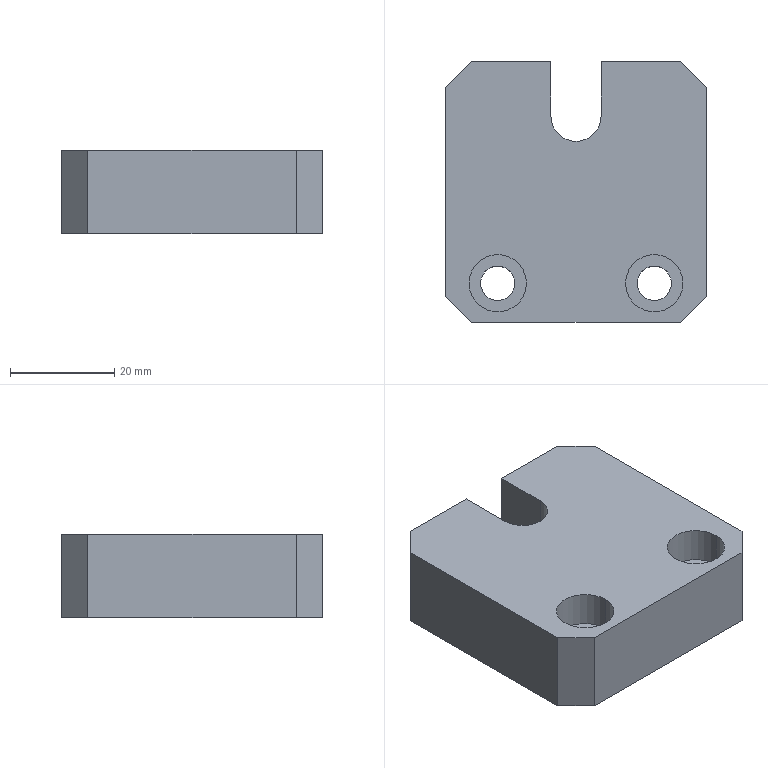Part | STEP file | PN_0017 | 1 solid | 24 faces | box 50 x 50 x 16 mm | volume 35086 mm3 | plane 15 | cylinder 9 | commonest cylinder face diameters 6.6 x4 11 x4 9.6 x1